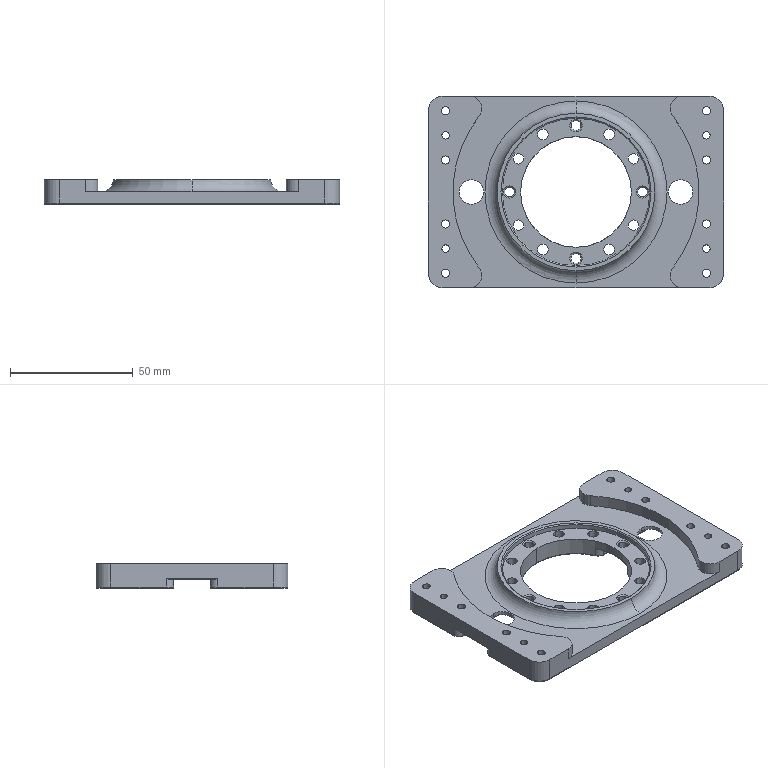NC program | NX | posted with a generic post | part box 120 x 78 x 10 mm
Lines 125 to 991 of 5508:
(ADAPTIVE_MILLING , TOOL : D10)
N212 T15 M6
N214 G54
N216 G17 G0 G90 X-71.209 Y-0.062 B0. C0. S9500 M3
N218 G43 Z30. H15
N220 Z-7.
N222 G94 G1 Z-10. F1000.
N224 X-70.428 Y-0.342 F3000.
N226 X-69.64 Y-0.598
N228 G3 X-68.562 Y-0.062 R1.017
N230 X-67.801 Y3.001 R8.28
N232 X-67.519 Y12.869 R111.643
N234 G1 X-67.514 Y15.119
N236 X-67.511 Y18.994
N238 X-67.51 Y32.619
N240 Y39.369
N242 X-67.509 Y39.494
N244 X-67.508 Y39.618
N246 G2 X-65.014 Y43.899 R5.714
N248 X-59.574 Y45.965 R12.318
N250 X-51.471 Y46.453 R57.403
N252 G1 X-50.471 Y46.463
N254 X-49.221 Y46.472
N256 X-47.471 Y46.479
N258 X-45.346 Y46.484
N260 X-41.721 Y46.487
N262 X-30.096 Y46.488
N264 X60.529
N266 X60.654 Y46.486
N268 X60.779 Y46.48
N270 X60.903 Y46.469
N272 G2 X65.069 Y43.765 R5.94
N274 X67.03 Y38.15 R13.153
N276 X67.463 Y29.542 R69.654
N278 G1 X67.472 Y28.292
N280 X67.479 Y26.667
N282 X67.484 Y24.417
N284 X67.487 Y20.667
N286 X67.488 Y8.917
N288 Y-39.458
N290 G2 X65.218 Y-43.724 R5.567
N292 X59.958 Y-45.896 R11.69
N294 X52.485 Y-46.438 R47.762
N296 X35.111 Y-46.488 R917.334
N298 G1 X-60.514
N300 X-60.639 Y-46.486
N302 X-60.764 Y-46.48
N304 X-60.889 Y-46.47
N306 G2 X-65.06 Y-43.775 R5.92
N308 X-67.027 Y-38.163 R13.09
N310 X-67.464 Y-29.305 R70.992
N312 G1 X-67.473 Y-28.055
N314 X-67.479 Y-26.43
N316 X-67.484 Y-24.18
N318 X-67.487 Y-20.305
N320 X-67.488 Y-7.305
N322 Y-3.805
N324 G2 X-66.99 Y1.418 R59.156
N326 G3 X-66.537 Y13.78 R127.385
N328 G1 X-66.53 Y15.655
N330 X-66.525 Y18.155
N332 X-66.522 Y22.28
N334 X-66.521 Y34.905
N336 Y36.405
N338 X-66.519 Y36.53
N340 G2 X-62.816 Y42.835 R7.66
N342 X-56.345 Y44.988 R15.672
N344 X-47.237 Y45.445 R77.787
N346 G1 X-45.987 Y45.456
N348 X-44.487 Y45.464
N350 X-42.612 Y45.47
N352 X-39.987 Y45.475
N354 X-34.987 Y45.477
N356 X10.638 Y45.478
N358 X57.388
N360 X57.638 Y45.475
N362 X57.763 Y45.471
N364 X57.888 Y45.465
N366 G2 X63.828 Y41.797 R7.663
N368 X65.948 Y35.576 R15.328
N370 X66.45 Y25.721 R77.207
N372 G1 X66.459 Y24.471
N374 X66.467 Y22.721
N376 X66.472 Y20.721
N378 X66.476 Y17.346
N380 X66.477 Y9.846
N382 X66.478 Y-36.404
N384 G2 X62.883 Y-42.766 R7.605
N386 X56.555 Y-44.952 R15.245
N388 X47.325 Y-45.444 R72.838
N390 G1 X46.2 Y-45.454
N392 X44.825 Y-45.462
N394 X42.95 Y-45.469
N396 X40.45 Y-45.474
N398 X36.075 Y-45.477
N400 X19.45 Y-45.478
N402 X-32.175
N404 X-32.925 Y-45.481
N406 X-34.05 Y-45.483
N408 X-34.925
N410 X-35.675 Y-45.485
N412 X-36.8
N414 X-37.175
N416 X-38.05 Y-45.487
N418 X-39.05 Y-45.486
N420 X-39.675 Y-45.485
N422 X-40.3 Y-45.487
N424 X-41.8
N426 X-42.8 Y-45.485
N428 X-43.55 Y-45.487
N430 X-44.55 Y-45.486
N432 X-44.925
N434 X-46.175 Y-45.489
N436 X-47.175 Y-45.487
N438 X-47.925 Y-45.488
N440 X-49.05 Y-45.487
N442 X-49.425
N444 X-50.55 Y-45.489
N446 X-51.925 Y-45.486
N448 G2 X-58.174 Y-45.452 R168.553
N450 X-63.981 Y-41.559 R7.806
N452 X-66.02 Y-35.048 R16.298
N454 X-66.452 Y-25.438 R86.279
N456 G1 X-66.46 Y-24.188
N458 X-66.467 Y-22.563
N460 X-66.472 Y-20.313
N462 X-66.476 Y-16.813
N464 X-66.477 Y-8.313
N466 Y-6.188
N468 G2 X-65.993 Y1.294 R100.923
N470 G3 X-65.547 Y15.783 R186.777
N472 G1 X-65.54 Y17.908
N474 X-65.535 Y20.783
N476 X-65.532 Y25.533
N478 X-65.531 Y33.408
N480 X-65.53 Y33.783
N482 X-65.528 Y33.908
N484 G2 X-60.818 Y41.902 R8.985
N486 G3 X-59.533 Y42.676 R12.441
N488 G2 X-55.89 Y43.985 R12.815
N490 X-42.858 Y44.45 R139.535
N492 G1 X-41.233 Y44.456
N494 X-38.858 Y44.462
N496 X-34.983 Y44.465
N498 X-25.983 Y44.467
N500 X54.767
N502 X55.017 Y44.465
N504 G2 X62.957 Y39.679 R8.935
N506 G3 X63.676 Y38.533 R14.031
N508 G2 X64.985 Y34.89 R12.815
N510 X65.442 Y22.983 R128.688
N512 G1 X65.451 Y21.358
N514 X65.458 Y19.358
N516 X65.463 Y16.733
N518 X65.466 Y12.233
N520 X65.467 Y-3.642
N522 Y-33.767
N524 G2 X60.675 Y-41.956 R8.962
N526 G3 X59.533 Y-42.676 R15.609
N528 G2 X55.89 Y-43.985 R12.815
N530 X43.608 Y-44.445 R132.262
N532 G1 X42.108 Y-44.453
N534 X39.983 Y-44.459
N536 X36.983 Y-44.464
N538 X31.608 Y-44.466
N540 X-10.267 Y-44.467
N542 X-29.142
N544 X-30.017 Y-44.472
N546 X-31.142 Y-44.474
N548 X-32.017 Y-44.475
N550 X-32.767 Y-44.478
N552 X-33.892 Y-44.48
N554 X-34.892
N556 X-35.767 Y-44.483
N558 X-36.517
N560 X-37.142 Y-44.482
N562 X-38.142 Y-44.485
N564 X-39.267 Y-44.483
N566 X-39.892 Y-44.482
N568 X-41.142 Y-44.486
N570 X-42.392 Y-44.484
N572 X-43.642 Y-44.488
N574 X-44.517 Y-44.487
N576 X-45.767 Y-44.488
N578 X-46.267 Y-44.489
N580 G2 X-55.641 Y-44.459 R647.854
N582 X-62.891 Y-39.797 R8.889
N584 G3 X-63.676 Y-38.533 R14.025
N586 G2 X-64.985 Y-34.89 R12.815
N588 X-65.442 Y-22.983 R129.141
N590 X-65.413 Y-5.359 R707.313
N592 G1 X-65.393 Y-4.859
N594 X-65.369 Y-4.36
N596 X-65.341 Y-3.86
N598 X-65.318 Y-3.486
N600 X-65.277 Y-2.863
N602 X-65.198 Y-1.74
N604 X-65.15 Y-1.076
N606 Y32.977
N608 X-65.148 Y33.023
N610 G2 X-64.458 Y36.856 R12.92
N612 X-61.129 Y41.568 R11.981
N614 G1 X-60.003 Y42.357
N616 X-59.533 Y42.676
N618 X-57.769 Y43.49
N620 X-55.89 Y43.985
N622 X-53.977 Y44.15
N624 X53.977
N626 X54.023 Y44.148
N628 G2 X57.856 Y43.458 R12.92
N630 X62.568 Y40.129 R11.981
N632 G1 X63.213 Y39.208
N634 X63.676 Y38.533
N636 X64.49 Y36.769
N638 X64.985 Y34.89
N640 X65.15 Y32.977
N642 Y-32.977
N644 X65.148 Y-33.023
N646 G2 X64.458 Y-36.856 R12.92
N648 X61.129 Y-41.568 R11.981
N650 G1 X60.208 Y-42.213
N652 X59.533 Y-42.676
N654 X57.769 Y-43.49
N656 X55.89 Y-43.985
N658 X53.977 Y-44.15
N660 X-53.977
N662 X-54.023 Y-44.148
N664 G2 X-57.856 Y-43.458 R12.92
N666 X-62.568 Y-40.129 R11.981
N668 G1 X-63.213 Y-39.208
N670 X-63.676 Y-38.533
N672 X-64.49 Y-36.769
N674 X-64.985 Y-34.89
N676 X-65.15 Y-32.977
N678 Y-0.977
N680 G3 X-66. Y0.021 R1.016
N682 G1 X-67.563 Y0.27
N684 Z-7.
N686 G0 Z30.
N688 X-2.465 Y-3.783
N690 Z3.
N692 G3 X-2.465 Y-3.783 Z2.506 I2.431 J3.787 F1000.
N694 X-2.465 Y-3.783 Z2.013 I2.431 J3.787
N696 X-2.465 Y-3.783 Z1.519 I2.431 J3.787
N698 X-2.465 Y-3.783 Z1.026 I2.431 J3.787
N700 X-2.465 Y-3.783 Z0.532 I2.431 J3.787
N702 X-2.465 Y-3.783 Z0.039 I2.431 J3.787
N704 X-2.465 Y-3.783 Z-0.455 I2.431 J3.787
N706 X-2.465 Y-3.783 Z-0.948 I2.431 J3.787
N708 X-2.465 Y-3.783 Z-1.442 I2.431 J3.787
N710 X-2.465 Y-3.783 Z-1.935 I2.431 J3.787
N712 X-2.465 Y-3.783 Z-2.429 I2.431 J3.787
N714 X-2.465 Y-3.783 Z-2.922 I2.431 J3.787
N716 X-2.465 Y-3.783 Z-3.416 I2.431 J3.787
N718 X-2.465 Y-3.783 Z-3.909 I2.431 J3.787
N720 X-2.465 Y-3.783 Z-4.403 I2.431 J3.787
N722 X-2.465 Y-3.783 Z-4.896 I2.431 J3.787
N724 X-2.465 Y-3.783 Z-5.39 I2.431 J3.787
N726 X-2.465 Y-3.783 Z-5.884 I2.431 J3.787
N728 X-2.465 Y-3.783 Z-6.377 I2.431 J3.787
N730 X-2.465 Y-3.783 Z-6.871 I2.431 J3.787
N732 X-2.465 Y-3.783 Z-7.364 I2.431 J3.787
N734 X-2.465 Y-3.783 Z-7.858 I2.431 J3.787
N736 X-2.465 Y-3.783 Z-8.351 I2.431 J3.787
N738 X-2.465 Y-3.783 Z-8.845 I2.431 J3.787
N740 X-2.465 Y-3.783 Z-9.338 I2.431 J3.787
N742 X-2.465 Y-3.783 Z-9.832 I2.431 J3.787
N744 X4.466 Y0.004 Z-10. R4.5
N746 X3.645 Y-2.601 R-4.501 F3000.
N748 X-1.026 Y4.875 R4.673
N750 X3.77 Y-3.237 R-4.977
N752 X-2. Y5.103 R5.196
N754 X3.648 Y-4.074 R-5.476
N756 X-2.758 Y5.328 R5.722
N758 X3.769 Y-4.665 R-5.998
N760 X-2.651 Y5.977 R6.259
N762 X4.213 Y-5.01 R-6.542
N764 X-2.93 Y6.46 R6.81
N766 X3.83 Y-5.983 R-7.099
N768 X-3.303 Y6.923 R7.384
N770 X4.115 Y-6.5 R-7.682
N772 X-4.147 Y7.154 R7.98
N774 X-7.164 Y-4.165 R8.283
N776 X4.154 Y-7.183 R8.283
N778 X7.359 Y4.537 R8.591
N780 X-4.405 Y7.716 R8.591
N782 X4.293 Y-7.812 R8.899
N784 X7.994 Y4.678 R9.211
N786 X-4.418 Y8.421 R9.211
N788 X4.181 Y-8.581 R9.528
N790 X-3.327 Y9.588 R9.846
N792 X-9.613 Y-3.348 R10.17
N794 X3.367 Y-9.619 R10.17
N796 X9.818 Y3.755 R10.5
N798 X-3.619 Y10.184 R10.5
N800 X3.099 Y-10.402 R10.831
N802 X10.603 Y3.491 R11.165
N804 X-3.226 Y11.014 R11.165
N806 X3.951 Y-10.836 R-11.506
N808 X-3.043 Y11.769 R11.845
N810 X2.74 Y-11.907 R12.187
N812 X-2.131 Y12.663 R12.53
N814 X1.717 Y-12.801 R12.878
N816 X0.082 Y13.524 R13.224
N818 X-1.641 Y-13.519 R13.568
N820 X7.034 Y12.276 R13.906
N822 X-11.521 Y-8.539 R14.225
N824 X14.57 Y-0.618 R14.512
N826 X-11.958 Y9.137 R14.781
N828 X5.86 Y-13.927 R15.086
N830 X-4.961 Y14.938 R15.425
N832 X0.939 Y-15.792 R15.777
N834 X7.354 Y14.612 R16.116
N836 X-14.214 Y-8.476 R16.423
N838 X16.752 Y-1.172 R16.71
N840 X-14.486 Y9.429 R17.01
N842 X-16.942 Y-3.511 R17.216
N844 X6.946 Y-15.878 R17.324
N846 X11.471 Y-13.01 R18.884
N848 X14.694 Y-9.216 R19.902
N850 X16.706 Y-4.663 R19.902
N852 X17.342 Y0.274 R19.902
N854 X16.55 Y5.189 R19.902
N856 X14.423 Y9.634 R19.954
N858 X9.191 Y14.71 R18.613
N860 X2.335 Y17.187 R18.613
N862 X-2.465 Y17.169 R19.795
N864 X-9.101 Y14.766 R18.57
N866 X-14.231 Y9.917 R18.57
N868 X-16.433 Y5.549 R19.967
N870 X-17.335 Y0.581 R19.925
N872 X-16.767 Y-4.437 R19.925
N874 G1 X-16.003 Y-6.688
N876 X-15.943 Y-6.831
N878 X-14.859 Y-8.946
N880 X-14.779 Y-9.079
N882 X-13.399 Y-11.014
N884 X-13.3 Y-11.133
N886 X-11.653 Y-12.847
N888 X-11.538 Y-12.951
N890 X-9.659 Y-14.406
N892 X-9.529 Y-14.492
N894 X-7.459 Y-15.659
N896 X-7.318 Y-15.725
N898 X-5.1 Y-16.578
N900 X-4.951 Y-16.623
N902 X-2.632 Y-17.144
N904 X-2.479 Y-17.166
N906 X-0.582 Y-17.309
N908 X0.295 Y-17.327
N910 X2.383 Y-17.18
N912 X2.534 Y-17.159
N914 X4.823 Y-16.661
N916 X4.97 Y-16.617
N918 X7.164 Y-15.796
N920 X7.303 Y-15.732
N922 X9.357 Y-14.604
N924 X9.485 Y-14.521
N926 G3 X9.617 Y-13.028 R1.014
N928 G1 X8.664 Y-12.001
N930 Z-7.
N932 G0 Z30.
(ADAPTIVE_MILLING_COPY , TOOL : D10)
N934 X-33.131 Y-24.065
N936 Z3.
N938 G3 X-33.131 Y-24.065 Z2.506 I-4.475 J0.47 F1000.
N940 X-33.131 Y-24.065 Z2.013 I-4.475 J0.47
N942 X-33.131 Y-24.065 Z1.519 I-4.475 J0.47
N944 X-33.131 Y-24.065 Z1.026 I-4.475 J0.47
N946 X-33.131 Y-24.065 Z0.532 I-4.475 J0.47
N948 X-33.131 Y-24.065 Z0.039 I-4.475 J0.47
N950 X-33.131 Y-24.065 Z-0.455 I-4.475 J0.47
N952 X-33.131 Y-24.065 Z-0.948 I-4.475 J0.47
N954 X-33.131 Y-24.065 Z-1.442 I-4.475 J0.47
N956 X-33.106 Y-23.595 Z-1.45 R4.5
N958 X-33.927 Y-26.2 R-4.501 F3000.
N960 X-38.598 Y-18.727 R4.669
N962 X-34.019 Y-27.064 R-4.976
N964 X-32.506 Y-22.377 R5.183
N966 X-33.226 Y-20.705 R3.085
N968 X-39.704 Y-18.519 R5.067
N970 X-42.849 Y-22.027 R5.312
N972 X-42.78 Y-25.023 R22.255
N974 X-39.117 Y-28.849 R5.073
N976 X-36.246 Y-28.786 R22.541
N978 X-31.904 Y-22.77 R5.556
N980 G1 X-31.938 Y-22.65
N982 X-31.985 Y-22.534
N984 X-32.026 Y-22.452
N986 X-33.2 Y-20.745
N988 X-33.226 Y-20.705
N990 X-33.41 Y-20.378
N992 G3 X-34.625 Y-18.655 R5.448
N994 X-38.251 Y-17.66 R5.029
N996 X-42.795 Y-20.559 R5.533
N998 X-42.849 Y-22.059 R7.011
N1000 X-41.423 Y-23.11 R1.103
N1002 G1 X-34.594 Y-20.988
N1004 G3 X-33.962 Y-19.398 R1.103
N1006 X-35.419 Y-17.74 R3.534
N1008 G1 X-35.537 Y-17.697
N1010 X-35.658 Y-17.667
N1012 X-35.781 Y-17.65
N1014 X-37.031
N1016 G3 X-37.353 Y-19.802 R1.1
N1018 G1 X-35.61 Y-20.336
N1020 G3 X-34.33 Y-18.744 R1.101
N1022 X-35.031 Y-17.795 R2.324
N1024 X-35.817 Y-17.65 R1.587
N1026 G1 X-38.001
N1028 G3 X-40.237 Y-17.792 R8.005
N1030 X-42.735 Y-19.566 R4.61
N1032 X-42.849 Y-20.84 R3.137
N1034 X-41.022 Y-21.665 R1.101
N1036 G1 X-38.649 Y-19.575
N1038 G3 X-39.376 Y-17.65 R1.101
N1040 X-42.113 Y-18.3 R4.193
N1042 X-42.849 Y-19.348 R1.499
N1044 G1 Y-19.973
N1046 G3 X-41.053 Y-20.825 R1.101
N1048 G1 X-39.555 Y-19.602
N1050 G3 X-40.251 Y-17.65 R1.101
N1052 X-42.191 Y-17.982 R3.488
N1054 X-42.849 Y-19.427 R1.38
N1056 X-41.01 Y-20.242 R1.101
N1058 G1 X-40.569 Y-19.847
N1060 X-40.142 Y-19.437
N1062 G3 X-41.001 Y-17.65 R1.101
N1064 X-42.342 Y-17.841 R2.517
N1066 X-42.848 Y-18.962 R1.196
N1068 X-40.34 Y-18.969 R1.254
N1070 X-41.626 Y-17.65 R1.291
N1072 X-42.845 Y-18.685 R1.088
N1074 G1 X-42.848 Y-18.712
N1076 X-42.849 Y-24.402
N1078 G3 X-42.568 Y-26.611 R4.987
N1080 X-40.573 Y-28.779 R4.737
N1082 X-39.025 Y-28.849 R5.766
N1084 X-38.307 Y-26.916 R1.101
N1086 G1 X-41.032 Y-24.569
N1088 G3 X-42.849 Y-25.402 R1.101
N1090 X-41.462 Y-28.701 R3.657
N1092 X-40.238 Y-28.849 R2.47
N1094 X-39.47 Y-26.961 R1.101
N1096 G1 X-40.982 Y-25.489
N1098 G3 X-42.85 Y-26.277 R1.101
N1100 X-42.113 Y-28.58 R2.908
N1102 X-40.972 Y-28.849 R1.576
N1104 X-40.162 Y-27.005 R1.101
N1106 G1 X-40.607 Y-26.514
N1108 X-41.068 Y-26.039
N1110 G3 X-42.85 Y-26.902 R1.101
N1112 X-42.529 Y-28.456 R2.337
N1114 X-41.393 Y-28.849 R1.303
N1116 X-40.812 Y-26.815 R1.101
N1118 G1 X-41.329 Y-26.511
N1120 G3 X-42.85 Y-27.527 R1.102
N1122 X-41.662 Y-28.849 R1.129
N1124 G1 X-36.867
N1126 G3 X-34.65 Y-28.602 R5.436
N1128 X-31.355 Y-23.679 R5.564
N1130 G1 X-31.503 Y-23.21
N1132 X-32.07 Y-22.387
N1134 G3 X-33.926 Y-22.456 R1.102
N1136 G1 X-36.692 Y-27.195
N1138 G3 X-35.742 Y-28.849 R1.102
N1140 X-32.136 Y-27.243 R4.02
N1142 X-30.914 Y-24.295 R4.977
N1144 X-31.51 Y-23.201 R2.616
N1146 X-33.335 Y-23.221 R1.102
N1148 G1 X-35.911 Y-27.146
N1150 G3 X-34.992 Y-28.849 R1.102
N1152 X-31.604 Y-27.343 R3.765
N1154 X-30.522 Y-24.745 R4.074
N1156 X-31.114 Y-23.752 R1.999
N1158 X-32.864 Y-23.828 R1.103
N1160 G1 X-35.146 Y-27.123
N1162 G3 X-34.242 Y-28.849 R1.101
N1164 X-30.996 Y-27.332 R3.596
N1166 X-30.157 Y-25.164 R3.345
N1168 X-30.745 Y-24.196 R2.049
N1170 X-32.506 Y-24.288 R1.103
N1172 G1 X-34.407 Y-27.139
N1174 G3 X-33.492 Y-28.85 R1.102
N1176 X-30.411 Y-27.289 R3.362
N1178 X-29.849 Y-25.428 R2.44
N1180 X-30.408 Y-24.601 R2.576
N1182 X-32.172 Y-24.699 R1.103
N1184 G1 X-33.785 Y-27.144
N1186 G3 X-32.867 Y-28.85 R1.102
N1188 X-29.5 Y-26.026 R3.139
N1190 X-30.025 Y-25.062 R1.692
N1192 X-31.777 Y-25.14 R1.103
N1194 G1 X-33.147 Y-27.125
N1196 G3 X-32.242 Y-28.85 R1.101
N1198 X-29.215 Y-26.464 R2.809
N1200 X-29.738 Y-25.408 R1.574
N1202 X-31.482 Y-25.476 R1.103
N1204 G1 X-32.64 Y-27.115
N1206 G3 X-31.742 Y-28.85 R1.101
N1208 X-28.962 Y-26.738 R2.482
N1210 X-29.481 Y-25.717 R1.593
N1212 X-31.234 Y-25.796 R1.103
N1214 G1 X-31.745 Y-26.528
N1216 X-32.234 Y-27.274
N1218 G3 X-31.242 Y-28.85 R1.102
N1220 X-28.74 Y-27.098 R2.241
N1222 X-29.212 Y-26.041 R1.426
N1224 X-30.968 Y-26.126 R1.103
N1226 G1 X-31.361 Y-26.696
N1228 X-31.736 Y-27.279
N1230 G3 X-30.742 Y-28.85 R1.102
N1232 X-28.534 Y-27.291 R1.943
N1234 X-28.972 Y-26.33 R1.228
N1236 X-31.73 Y-27.471 R1.583
N1238 X-30.242 Y-28.85 R1.498
N1240 X-28.35 Y-27.327 R1.614
N1242 X-28.872 Y-26.433 R1.405
N1244 X-29.867 Y-28.85 R-1.414
N1246 X-28.184 Y-27.575 R1.44
N1248 X-28.621 Y-26.685 R1.24
N1250 X-30.046 Y-28.723 R-1.261
N1252 G1 X-29.776 Y-28.814
N1254 X-29.492 Y-28.85
N1256 G3 X-28.129 Y-27.303 R1.188
N1258 X-28.492 Y-26.815 R2.354
N1260 X-30.414 Y-27.929 R1.152
N1262 X-29.242 Y-28.85 R1.213
N1264 X-28.359 Y-26.949 R1.086
N1266 X-28.954 Y-26.659 R1.05
N1268 G1 X-32.278 Y-26.261
N1270 Z1.55
N1272 G0 Z30.
N1274 X-33.131 Y23.123
N1276 Z3.
N1278 G3 X-33.131 Y23.123 Z2.506 I-4.475 J0.47 F1000.
N1280 X-33.131 Y23.123 Z2.013 I-4.475 J0.47
N1282 X-33.131 Y23.123 Z1.519 I-4.475 J0.47
N1284 X-33.131 Y23.123 Z1.026 I-4.475 J0.47
N1286 X-33.131 Y23.123 Z0.532 I-4.475 J0.47
N1288 X-33.131 Y23.123 Z0.039 I-4.475 J0.47
N1290 X-33.131 Y23.123 Z-0.455 I-4.475 J0.47
N1292 X-33.131 Y23.123 Z-0.948 I-4.475 J0.47
N1294 X-33.131 Y23.123 Z-1.442 I-4.475 J0.47
N1296 X-33.107 Y23.594 Z-1.45 R4.5
N1298 X-33.928 Y20.988 R-4.501 F3000.
N1300 X-38.904 Y28.389 R4.675
N1302 X-34.02 Y20.124 R-4.976
N1304 X-32.507 Y24.812 R5.181
N1306 X-36.156 Y28.85 R4.96
N1308 X-39.027 Y28.775 R20.168
N1310 X-42.85 Y25.138 R5.086
N1312 X-42.78 Y22.142 R21.345
N1314 X-34.941 Y18.783 R5.336
N1316 X-33.848 Y19.601 R3.762
N1318 G2 X-32.384 Y22.003 R52.002
N1320 G3 X-34.684 Y28.791 R5.307
N1322 X-36.2 Y28.85 R6.429
N1324 G1 X-38.281
N1326 G3 X-40.384 Y28.661 R5.874
N1328 X-42.782 Y26.571 R4.688
N1330 X-42.85 Y25.03 R5.872
N1332 X-40.917 Y24.312 R1.101
N1334 G1 X-38.573 Y27.032
N1336 G3 X-39.406 Y28.85 R1.101
N1338 X-42.704 Y27.46 R3.66
N1340 X-42.85 Y26.235 R2.498
N1342 X-40.992 Y25.438 R1.101
N1344 G1 X-39.399 Y26.953
N1346 G3 X-40.156 Y28.85 R1.101
N1348 X-42.497 Y28.203 R3.165
N1350 X-42.85 Y26.976 R1.486
N1352 X-41.006 Y26.166 R1.101
N1354 G1 X-40.517 Y26.608
N1356 X-40.043 Y27.068
N1358 G3 X-40.906 Y28.85 R1.101
N1360 X-42.461 Y28.529 R2.327
N1362 X-42.85 Y27.394 R1.307
N1364 X-40.812 Y26.819 R1.101
N1366 G1 X-40.513 Y27.335
N1368 G3 X-41.531 Y28.85 R1.102
N1370 X-42.85 Y27.663 R1.127
N1372 G1 Y22.763
N1374 G3 X-42.559 Y20.555 R4.859
N1376 X-38.626 Y17.651 R5.302
N1378 X-35.772 Y17.868 R9.765
N1380 X-34.41 Y18.603 R2.477
N1382 G1 X-33.796 Y19.692
N1384 G3 X-34.519 Y21.306 R1.103
N1386 G1 X-41.515 Y22.837
N1388 G3 X-42.85 Y21.763 R1.103
N1390 X-41.086 Y18.124 R3.899
N1392 X-40.117 Y17.651 R2.177
N1394 G1 X-38.617
N1396 G3 X-37.973 Y19.642 R1.101
N1398 G1 X-41.106 Y21.904
N1400 G3 X-42.85 Y21.013 R1.101
N1402 X-41.233 Y17.728 R3.372
N1404 X-40.04 Y17.651 R3.859
N1406 X-39.311 Y19.575 R1.101
N1408 G1 X-41.021 Y21.087
N1410 G3 X-42.85 Y20.263 R1.101
N1412 X-42.015 Y17.876 R2.878
N1414 X-40.807 Y17.651 R1.864
N1416 X-40.053 Y19.552 R1.101
N1418 G1 X-40.587 Y20.063
N1420 X-41.139 Y20.553
N1422 G3 X-42.85 Y19.638 R1.102
N1424 X-42.535 Y18.078 R2.441
N1426 X-41.375 Y17.651 R1.283
N1428 X-40.745 Y19.653 R1.101
N1430 G1 X-41.268 Y20.002
N1432 G3 X-42.85 Y19.013 R1.102
N1434 X-41.663 Y17.651 R1.144
N1436 G1 X-37.126 Y17.65
N1438 G3 X-35.257 Y17.725 R9.196
N1440 X-34.396 Y18.627 R1.572
N1442 X-36.152 Y19.925 R1.1
N1444 G1 X-36.656 Y19.375
N1446 G3 X-35.751 Y17.65 R1.101
N1448 X-34.66 Y18.167 R1.139
N1450 G1 X-33.2 Y20.746
N1452 X-32.633 Y21.57
N1454 G3 X-31.591 Y23.541 R5.243
N1456 X-33.648 Y28.721 R5.31
N1458 X-34.957 Y28.85 R2.97
N1460 X-35.962 Y27.304 R1.102
N1462 G1 X-33.906 Y22.674
N1464 G3 X-31.995 Y22.496 R1.102
N1466 X-31.347 Y26.381 R3.914
N1468 X-32.92 Y28.725 R4.392
N1470 X-34.095 Y28.85 R2.636
N1472 X-35.115 Y27.338 R1.102
N1474 G1 X-33.495 Y23.326
N1476 G3 X-31.569 Y23.114 R1.102
N1478 X-30.945 Y26.673 R3.636
N1480 X-32.275 Y28.728 R3.541
N1482 X-33.442 Y28.85 R2.666
N1484 X-34.459 Y27.331 R1.102
N1486 G1 X-33.059 Y23.936
N1488 G3 X-31.196 Y23.652 R1.102
N1490 X-30.461 Y26.558 R3.14
N1492 X-31.639 Y28.697 R3.338
N1494 X-32.739 Y28.85 R2.117
N1496 X-33.782 Y27.398 R1.102
N1498 G1 X-32.765 Y24.388
N1500 G3 X-30.877 Y24.037 R1.102
N1502 X-30.206 Y27.292 R3.153
N1504 X-31.267 Y28.77 R2.221
N1506 X-32.221 Y28.85 R2.914
N1508 X-33.271 Y27.423 R1.103
N1510 G1 X-32.454 Y24.797
N1512 G3 X-30.557 Y24.421 R1.102
N1514 X-30.498 Y28.599 R2.996
N1516 X-31.613 Y28.85 R1.596
N1518 X-32.671 Y27.449 R1.103
N1520 G1 X-32.062 Y25.305
N1522 G3 X-30.158 Y24.902 R1.101
N1524 X-30.1 Y28.619 R2.645
N1526 X-31.19 Y28.85 R1.629
N1528 X-32.247 Y27.446 R1.103
N1530 G1 X-31.742 Y25.686
N1532 G3 X-29.838 Y25.287 R1.101
N1534 X-29.651 Y28.563 R2.381
N1536 X-30.695 Y28.85 R1.391
N1538 X-31.764 Y27.494 R1.103
N1540 G1 X-31.585 Y26.72
N1542 X-31.381 Y25.953
N1544 G3 X-29.519 Y25.671 R1.102
N1546 X-29.345 Y28.589 R2.067
N1548 X-30.348 Y28.85 R1.404
N1550 X-31.4 Y27.429 R1.103
N1552 G1 X-31.227 Y26.845
N1554 X-31.03 Y26.269
N1556 G3 X-29.199 Y26.056 R1.102
N1558 X-29.017 Y28.557 R1.797
N1560 X-30.068 Y28.85 R1.386
N1562 X-30.852 Y26.179 R1.454
N1564 X-28.939 Y26.366 R1.516
N1566 X-28.891 Y28.658 R1.471
N1568 X-29.804 Y28.85 R1.513
N1570 X-30.369 Y26.274 R1.353
N1572 X-28.763 Y26.543 R1.407
N1574 X-28.71 Y28.683 R1.314
N1576 X-29.456 Y28.85 R1.439
N1578 X-30.19 Y26.725 R1.192
N1580 X-28.498 Y26.809 R1.263
N1582 X-29.292 Y28.85 R1.13
N1584 X-30.022 Y26.978 R1.083
N1586 X-28.322 Y26.986 R1.21
N1588 X-29.148 Y28.85 R1.072
N1590 X-29.831 Y28.584 R1.04
N1592 G1 X-32.261 Y26.35
N1594 Z1.55
N1596 G0 Z30.
N1598 X42.074 Y23.129
N1600 Z3.
N1602 G3 X42.074 Y23.129 Z2.506 I-4.475 J0.47 F1000.
N1604 X42.074 Y23.129 Z2.013 I-4.475 J0.47
N1606 X42.074 Y23.129 Z1.519 I-4.475 J0.47
N1608 X42.074 Y23.129 Z1.026 I-4.475 J0.47
N1610 X42.074 Y23.129 Z0.532 I-4.475 J0.47
N1612 X42.074 Y23.129 Z0.039 I-4.475 J0.47
N1614 X42.074 Y23.129 Z-0.455 I-4.475 J0.47
N1616 X42.074 Y23.129 Z-0.948 I-4.475 J0.47
N1618 X42.074 Y23.129 Z-1.442 I-4.475 J0.47
N1620 X42.099 Y23.599 Z-1.45 R4.5
N1622 X41.278 Y20.993 R-4.501 F3000.
N1624 X36.607 Y28.469 R4.67
N1626 X41.185 Y20.129 R-4.977
N1628 X42.699 Y24.816 R5.178
N1630 X39.068 Y28.85 R4.961
N1632 X36.198 Y28.783 R21.505
N1634 X32.396 Y21.913 R5.252
N1636 X33.843 Y19.768 R153.548
N1638 X40.994 Y19.255 R5.296
N1640 X42.823 Y21.582 R5.437
N1642 X42.8 Y25.733 R37.492
N1644 X40.45 Y28.803 R4.427
N1646 X38.959 Y28.85 R8.449
N1648 G1 X36.818
N1650 G3 X34.607 Y28.576 R5.077
N1652 X31.609 Y23.143 R5.304
N1654 X32.416 Y21.884 R7.922
N1656 X34.315 Y22.035 R1.102
N1658 G1 X36.811 Y27.277
N1660 G3 X35.818 Y28.85 R1.102
N1662 X32.16 Y27.125 R3.904
N1664 X31.079 Y23.996 R4.973
N1666 X31.721 Y22.893 R3.546
N1668 X33.592 Y22.989 R1.102
N1670 G1 X35.908 Y27.222
N1672 G3 X34.943 Y28.85 R1.102
N1674 X31.787 Y27.406 R3.556
N1676 X30.649 Y24.567 R4.372
N1678 X31.225 Y23.614 R2.064
N1680 X33.029 Y23.686 R1.102
N1682 G1 X35.246 Y27.158
N1684 G3 X34.318 Y28.85 R1.102
N1686 X31.18 Y27.384 R3.487
N1688 X30.271 Y24.987 R3.496
N1690 X30.859 Y24.058 R2.206
N1692 X32.621 Y24.152 R1.103
N1694 G1 X34.609 Y27.141
N1696 G3 X33.693 Y28.85 R1.102
N1698 X30.587 Y27.34 R3.368
N1700 X29.928 Y25.374 R2.791
N1702 X30.502 Y24.488 R2.301
N1704 X32.261 Y24.577 R1.103
N1706 G1 X33.981 Y27.136
N1708 G3 X33.068 Y28.85 R1.102
N1710 X29.583 Y25.976 R3.245
N1712 X30.181 Y24.874 R1.82
N1714 X31.949 Y24.976 R1.103
N1716 G1 X33.365 Y27.15
N1718 G3 X32.443 Y28.85 R1.102
N1720 X29.292 Y26.297 R2.89
N1722 X29.811 Y25.319 R1.642
N1724 X31.571 Y25.409 R1.103
N1726 G1 X32.731 Y27.137
N1728 G3 X31.818 Y28.85 R1.102
N1730 X29.032 Y26.583 R2.508
N1732 X29.556 Y25.626 R1.696
N1734 X31.327 Y25.733 R1.103
N1736 G1 X32.243 Y27.154
N1738 G3 X31.318 Y28.85 R1.102
N1740 X28.795 Y26.954 R2.249
N1742 X29.316 Y25.916 R1.582
N1744 X31.114 Y26.067 R1.102
N1746 G1 X31.491 Y26.706
N1748 X31.846 Y27.358
N1750 G3 X30.818 Y28.85 R1.102
N1752 X28.583 Y27.162 R1.955
N1754 X29.051 Y26.234 R1.4
N1756 X30.874 Y26.431 R1.102
N1758 G1 X31.127 Y26.913
N1760 X31.362 Y27.404
N1762 G3 X30.318 Y28.85 R1.102
N1764 X28.392 Y27.331 R1.674
N1766 X28.926 Y26.379 R1.386
N1768 X29.943 Y28.85 R-1.446
N1770 X28.226 Y27.464 R1.462
N1772 X28.664 Y26.642 R1.279
N1774 X29.568 Y28.85 R-1.291
N1776 X28.144 Y27.32 R1.228
N1778 X28.518 Y26.789 R1.823
N1780 X30.37 Y28.244 R1.187
N1782 X29.318 Y28.85 R1.229
N1784 X28.358 Y26.949 R1.105
N1786 X30.112 Y28.082 R1.07
N1788 X28.899 Y28.834 R1.133
N1790 X28.178 Y27.158 R1.05
N1792 G2 X33.409 Y20.379 R40.131
N1794 G3 X34.621 Y18.653 R5.495
N1796 X38.231 Y17.66 R5.009
N1798 X42.776 Y20.377 R5.723
N1800 X42.85 Y21.812 R5.012
N1802 X41.459 Y22.873 R1.103
N1804 G1 X34.629 Y20.999
N1806 G3 X33.961 Y19.399 R1.103
N1808 X35.418 Y17.74 R3.542
N1810 G1 X35.536 Y17.698
N1812 X35.657 Y17.668
N1814 X35.779 Y17.651
N1816 X37.029 Y17.65
N1818 G3 X37.351 Y19.802 R1.1
N1820 G1 X35.61 Y20.336
N1822 G3 X34.329 Y18.745 R1.101
N1824 X35.03 Y17.796 R2.325
N1826 X35.816 Y17.651 R1.587
N1828 G1 X37.981 Y17.65
N1830 G3 X40.22 Y17.775 R8.905
N1832 X42.744 Y19.504 R4.374
N1834 X42.85 Y20.761 R3.245
N1836 X41.042 Y21.604 R1.101
N1838 G1 X38.649 Y19.592
N1840 G3 X39.356 Y17.65 R1.101
N1842 X41.675 Y18.002 R4.694
N1844 X42.812 Y19.096 R1.976
N1846 X42.85 Y19.92 R10.15
N1848 X41.043 Y20.763 R1.101
N1850 G1 X39.649 Y19.593
N1852 G3 X40.356 Y17.65 R1.101
N1854 X42.287 Y18.01 R3.253
N1856 X42.85 Y19.398 R1.385
N1858 X40.97 Y20.173 R1.101
N1860 G1 X40.585 Y19.79
N1862 X40.214 Y19.394
N1864 G3 X41.106 Y17.65 R1.101
N1866 X42.428 Y17.892 R2.029
N1868 X42.85 Y18.963 R1.229
N1870 X40.51 Y19.223 R1.186
N1872 X41.731 Y17.65 R1.263
N1874 X42.83 Y18.562 R1.064
N1876 G1 X42.85 Y18.713
N1878 Y25.236
N1880 G3 X42.229 Y27.853 R3.977
N1882 X41.001 Y28.844 R1.971
N1884 G1 X40.956 Y28.85
N1886 X40.206
N1888 G3 X39.405 Y26.996 R1.101
N1890 G1 X40.949 Y25.356
N1892 G3 X42.85 Y26.111 R1.101
N1894 X42.126 Y28.547 R3.154
N1896 X40.95 Y28.85 R1.532
N1898 X40.132 Y27.014 R1.101
N1900 G1 X40.587 Y26.501
N1902 X41.061 Y26.004
N1904 G3 X42.85 Y26.861 R1.101
N1906 X42.542 Y28.422 R2.465
N1908 X41.381 Y28.85 R1.283
N1910 X40.74 Y26.856 R1.101
N1912 G1 X41.257 Y26.502
N1914 G3 X42.85 Y27.486 R1.102
N1916 X41.663 Y28.85 R1.145
N1918 X40.701 Y28.149 R1.017
N1920 G1 X40.122 Y26.35
N1922 Z1.55
N1924 G0 Z30.
N1926 X42.071 Y-24.076
N1928 Z3.
N1930 G3 X42.071 Y-24.076 Z2.506 I-4.475 J0.47 F1000.
N1932 X42.071 Y-24.076 Z2.013 I-4.475 J0.47